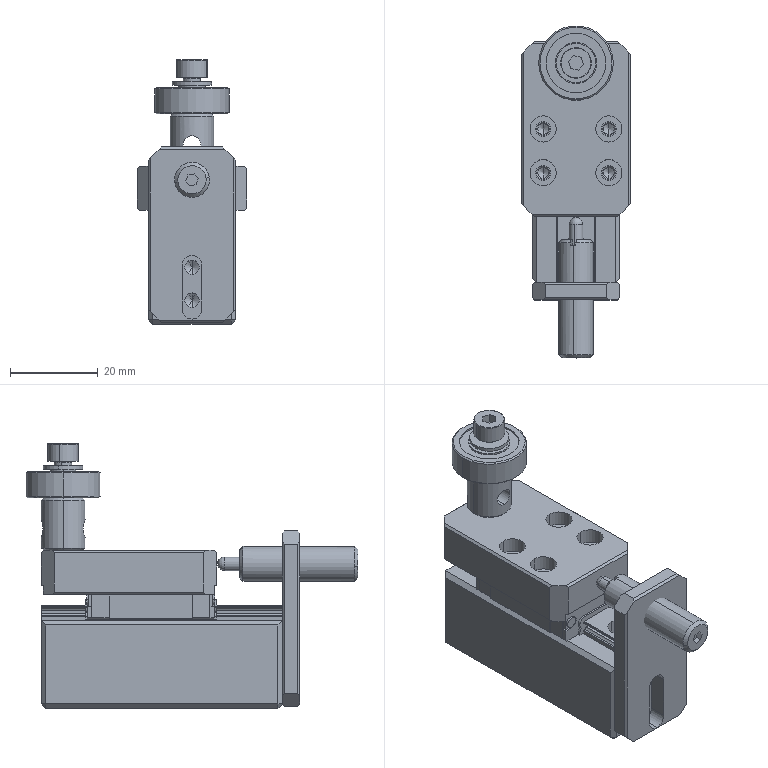Part | SolidWorks | 11 solids | 523 faces | box 25 x 75.736 x 60.345 mm | volume 39724 mm3 | plane 317 | cylinder 155 | cone 46 | torus 4 | sphere 1 | commonest cylinder face diameters 6 x18 2.2 x16 2.5 x14 3 x10 2.1 x8 2.459 x8